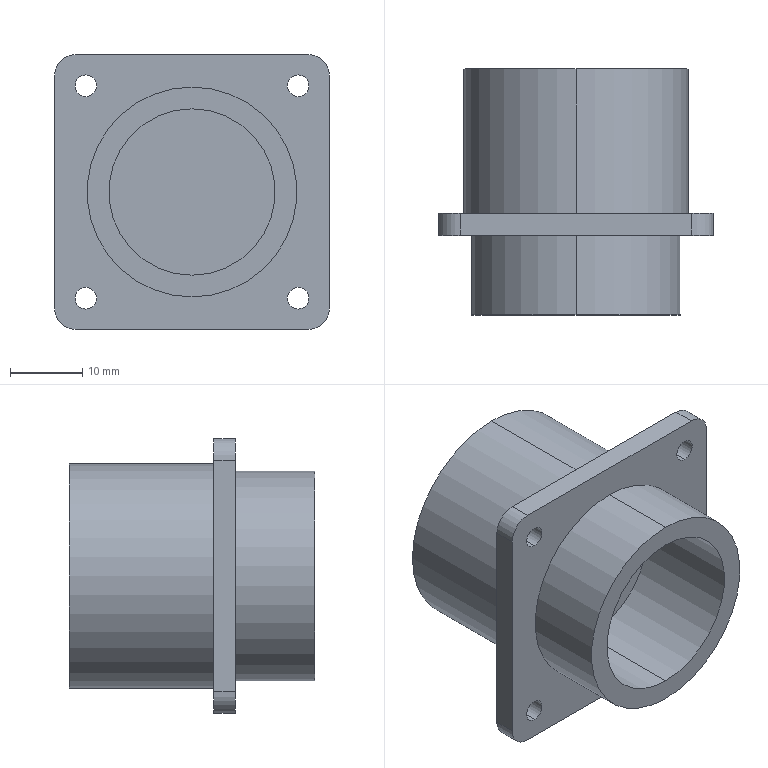Part | STEP file | 15050037_-3350001 | 1 solid | 102 faces | box 38 x 34 x 38 mm | volume 10767 mm3 | cylinder 55 | spline 34 | plane 13 | commonest cylinder face diameters 1.8 x34 3 x8 6 x4 27 x3 23 x2 29 x2